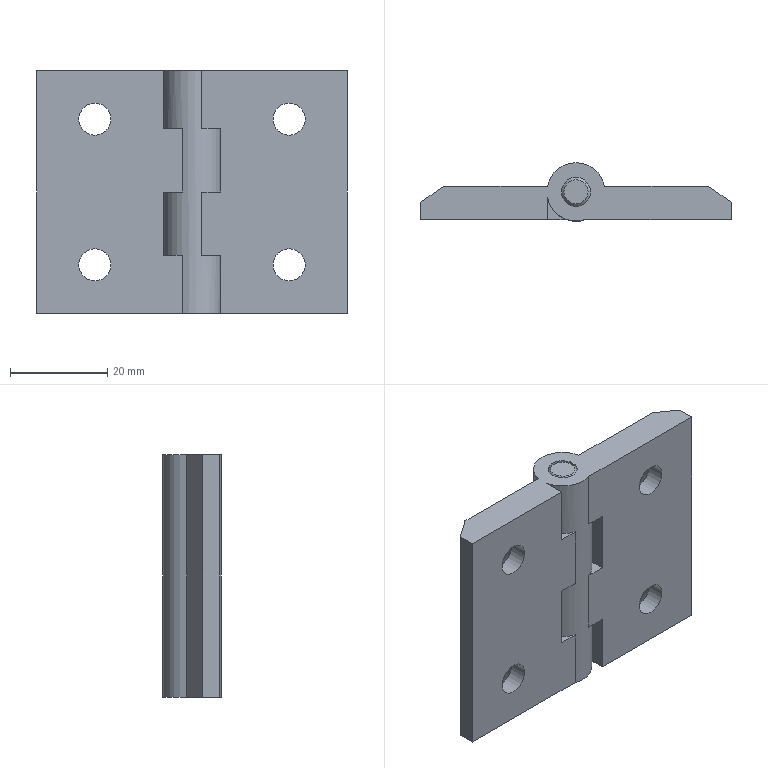Part | STEP file | 40-1-2-SOLID1_id370_x_t | 1 solid | 36 faces | box 64 x 12 x 50 mm | volume 21436 mm3 | plane 22 | cylinder 8 | cone 6 | commonest cylinder face diameters 6.6 x4 6 x2 12 x2
STEP:
#1=CARTESIAN_POINT('',(1872.,280.,-110.));
#2=VERTEX_POINT('',#1);
#3=CARTESIAN_POINT('',(1864.11,284.514,-110.));
#4=VERTEX_POINT('',#3);
#5=CARTESIAN_POINT('',(1870.,285.657,-110.));
#6=DIRECTION('',(0.,0.,-1.));
#7=DIRECTION('',(-1.,0.,0.));
#8=AXIS2_PLACEMENT_3D('',#5,#6,#7);
#9=CIRCLE('',#8,6.);
#10=EDGE_CURVE('',#2,#4,#9,.T.);
#11=ORIENTED_EDGE('',*,*,#10,.T.);
#12=CARTESIAN_POINT('',(1864.11,284.514,-122.));
#13=VERTEX_POINT('',#12);
#14=CARTESIAN_POINT('',(1864.11,284.514,-160.));
#15=DIRECTION('',(0.,0.,-1.));
#16=VECTOR('',#15,1.);
#17=LINE('',#14,#16);
#18=EDGE_CURVE('',#4,#13,#17,.T.);
#19=ORIENTED_EDGE('',*,*,#18,.T.);
#20=CARTESIAN_POINT('',(1868.,280.,-122.));
#21=VERTEX_POINT('',#20);
#22=CARTESIAN_POINT('',(1870.,285.657,-122.));
#23=DIRECTION('',(0.,0.,-1.));
#24=DIRECTION('',(1.,0.,0.));
#25=AXIS2_PLACEMENT_3D('',#22,#23,#24);
#26=CIRCLE('',#25,6.);
#27=EDGE_CURVE('',#21,#13,#26,.T.);
#28=ORIENTED_EDGE('',*,*,#27,.F.);
#29=CARTESIAN_POINT('',(1868.,280.,-135.));
#30=VERTEX_POINT('',#29);
#31=CARTESIAN_POINT('',(1868.,280.,-110.));
#32=DIRECTION('',(0.,0.,1.));
#33=VECTOR('',#32,1.);
#34=LINE('',#31,#33);
#35=EDGE_CURVE('',#30,#21,#34,.T.);
#36=ORIENTED_EDGE('',*,*,#35,.F.);
#37=CARTESIAN_POINT('',(1864.11,284.514,-135.));
#38=VERTEX_POINT('',#37);
#39=CARTESIAN_POINT('',(1870.,285.657,-135.));
#40=DIRECTION('',(0.,0.,-1.));
#41=DIRECTION('',(1.,0.,0.));
#42=AXIS2_PLACEMENT_3D('',#39,#40,#41);
#43=CIRCLE('',#42,6.);
#44=EDGE_CURVE('',#30,#38,#43,.T.);
#45=ORIENTED_EDGE('',*,*,#44,.T.);
#46=CARTESIAN_POINT('',(1864.11,284.514,-148.));
#47=VERTEX_POINT('',#46);
#48=CARTESIAN_POINT('',(1864.11,284.514,-160.));
#49=DIRECTION('',(0.,0.,1.));
#50=VECTOR('',#49,1.);
#51=LINE('',#48,#50);
#52=EDGE_CURVE('',#47,#38,#51,.T.);
#53=ORIENTED_EDGE('',*,*,#52,.F.);
#54=CARTESIAN_POINT('',(1868.,280.,-148.));
#55=VERTEX_POINT('',#54);
#56=CARTESIAN_POINT('',(1870.,285.657,-148.));
#57=DIRECTION('',(0.,0.,-1.));
#58=DIRECTION('',(-1.,0.,0.));
#59=AXIS2_PLACEMENT_3D('',#56,#57,#58);
#60=CIRCLE('',#59,6.);
#61=EDGE_CURVE('',#55,#47,#60,.T.);
#62=ORIENTED_EDGE('',*,*,#61,.F.);
#63=CARTESIAN_POINT('',(1868.,280.,-160.));
#64=VERTEX_POINT('',#63);
#65=CARTESIAN_POINT('',(1868.,280.,-110.));
#66=DIRECTION('',(0.,0.,1.));
#67=VECTOR('',#66,1.);
#68=LINE('',#65,#67);
#69=EDGE_CURVE('',#64,#55,#68,.T.);
#70=ORIENTED_EDGE('',*,*,#69,.F.);
#71=CARTESIAN_POINT('',(1875.89,284.514,-160.));
#72=VERTEX_POINT('',#71);
#73=CARTESIAN_POINT('',(1870.,285.657,-160.));
#74=DIRECTION('',(0.,0.,1.));
#75=DIRECTION('',(1.,0.,0.));
#76=AXIS2_PLACEMENT_3D('',#73,#74,#75);
#77=CIRCLE('',#76,6.);
#78=EDGE_CURVE('',#64,#72,#77,.T.);
#79=ORIENTED_EDGE('',*,*,#78,.T.);
#80=CARTESIAN_POINT('',(1875.89,284.514,-148.));
#81=VERTEX_POINT('',#80);
#82=CARTESIAN_POINT('',(1875.89,284.514,-110.));
#83=DIRECTION('',(0.,0.,-1.));
#84=VECTOR('',#83,1.);
#85=LINE('',#82,#84);
#86=EDGE_CURVE('',#81,#72,#85,.T.);
#87=ORIENTED_EDGE('',*,*,#86,.F.);
#88=CARTESIAN_POINT('',(1872.,280.,-148.));
#89=VERTEX_POINT('',#88);
#90=CARTESIAN_POINT('',(1870.,285.657,-148.));
#91=DIRECTION('',(0.,0.,1.));
#92=DIRECTION('',(1.,0.,0.));
#93=AXIS2_PLACEMENT_3D('',#90,#91,#92);
#94=CIRCLE('',#93,6.);
#95=EDGE_CURVE('',#89,#81,#94,.T.);
#96=ORIENTED_EDGE('',*,*,#95,.F.);
#97=CARTESIAN_POINT('',(1872.,280.,-135.));
#98=VERTEX_POINT('',#97);
#99=CARTESIAN_POINT('',(1872.,280.,-160.));
#100=DIRECTION('',(0.,0.,1.));
#101=VECTOR('',#100,1.);
#102=LINE('',#99,#101);
#103=EDGE_CURVE('',#89,#98,#102,.T.);
#104=ORIENTED_EDGE('',*,*,#103,.T.);
#105=CARTESIAN_POINT('',(1875.89,284.514,-135.));
#106=VERTEX_POINT('',#105);
#107=CARTESIAN_POINT('',(1870.,285.657,-135.));
#108=DIRECTION('',(0.,0.,1.));
#109=DIRECTION('',(-1.,0.,0.));
#110=AXIS2_PLACEMENT_3D('',#107,#108,#109);
#111=CIRCLE('',#110,6.);
#112=EDGE_CURVE('',#98,#106,#111,.T.);
#113=ORIENTED_EDGE('',*,*,#112,.T.);
#114=CARTESIAN_POINT('',(1875.89,284.514,-122.));
#115=VERTEX_POINT('',#114);
#116=CARTESIAN_POINT('',(1875.89,284.514,-110.));
#117=DIRECTION('',(0.,0.,1.));
#118=VECTOR('',#117,1.);
#119=LINE('',#116,#118);
#120=EDGE_CURVE('',#106,#115,#119,.T.);
#121=ORIENTED_EDGE('',*,*,#120,.T.);
#122=CARTESIAN_POINT('',(1872.,280.,-122.));
#123=VERTEX_POINT('',#122);
#124=CARTESIAN_POINT('',(1870.,285.657,-122.));
#125=DIRECTION('',(0.,0.,1.));
#126=DIRECTION('',(1.,0.,0.));
#127=AXIS2_PLACEMENT_3D('',#124,#125,#126);
#128=CIRCLE('',#127,6.);
#129=EDGE_CURVE('',#123,#115,#128,.T.);
#130=ORIENTED_EDGE('',*,*,#129,.F.);
#131=CARTESIAN_POINT('',(1872.,280.,-160.));
#132=DIRECTION('',(0.,0.,1.));
#133=VECTOR('',#132,1.);
#134=LINE('',#131,#133);
#135=EDGE_CURVE('',#123,#2,#134,.T.);
#136=ORIENTED_EDGE('',*,*,#135,.T.);
#137=EDGE_LOOP('',(#11,#19,#28,#36,#45,#53,#62,#70,#79,#87,#96,#104,#113,#121,#130,#136));
#138=FACE_OUTER_BOUND('',#137,.T.);
#139=CARTESIAN_POINT('',(1870.,285.657,-160.));
#140=DIRECTION('',(0.,0.,1.));
#141=DIRECTION('',(-1.,0.,0.));
#142=AXIS2_PLACEMENT_3D('',#139,#140,#141);
#143=CYLINDRICAL_SURFACE('',#142,6.);
#144=ADVANCED_FACE('',(#138),#143,.T.);
#145=CARTESIAN_POINT('',(1864.11,286.8,-160.));
#146=VERTEX_POINT('',#145);
#147=CARTESIAN_POINT('',(1864.11,286.8,-110.));
#148=VERTEX_POINT('',#147);
#149=CARTESIAN_POINT('',(1864.11,286.8,-110.));
#150=DIRECTION('',(0.,0.,1.));
#151=VECTOR('',#150,1.);
#152=LINE('',#149,#151);
#153=EDGE_CURVE('',#146,#148,#152,.T.);
#154=ORIENTED_EDGE('',*,*,#153,.T.);
#155=CARTESIAN_POINT('',(1875.89,286.8,-110.));
#156=VERTEX_POINT('',#155);
#157=CARTESIAN_POINT('',(1870.,285.657,-110.));
#158=DIRECTION('',(0.,0.,-1.));
#159=DIRECTION('',(-1.,0.,0.));
#160=AXIS2_PLACEMENT_3D('',#157,#158,#159);
#161=CIRCLE('',#160,6.);
#162=EDGE_CURVE('',#148,#156,#161,.T.);
#163=ORIENTED_EDGE('',*,*,#162,.T.);
#164=CARTESIAN_POINT('',(1875.89,286.8,-160.));
#165=VERTEX_POINT('',#164);
#166=CARTESIAN_POINT('',(1875.89,286.8,-160.));
#167=DIRECTION('',(0.,0.,1.));
#168=VECTOR('',#167,1.);
#169=LINE('',#166,#168);
#170=EDGE_CURVE('',#165,#156,#169,.T.);
#171=ORIENTED_EDGE('',*,*,#170,.F.);
#172=CARTESIAN_POINT('',(1870.,285.657,-160.));
#173=DIRECTION('',(0.,0.,1.));
#174=DIRECTION('',(1.,0.,0.));
#175=AXIS2_PLACEMENT_3D('',#172,#173,#174);
#176=CIRCLE('',#175,6.);
#177=EDGE_CURVE('',#165,#146,#176,.T.);
#178=ORIENTED_EDGE('',*,*,#177,.T.);
#179=EDGE_LOOP('',(#154,#163,#171,#178));
#180=FACE_OUTER_BOUND('',#179,.T.);
#181=CARTESIAN_POINT('',(1870.,285.657,-160.));
#182=DIRECTION('',(0.,0.,1.));
#183=DIRECTION('',(-1.,0.,0.));
#184=AXIS2_PLACEMENT_3D('',#181,#182,#183);
#185=CYLINDRICAL_SURFACE('',#184,6.);
#186=ADVANCED_FACE('',(#180),#185,.T.);
#187=CARTESIAN_POINT('',(1875.89,280.,-122.));
#188=VERTEX_POINT('',#187);
#189=CARTESIAN_POINT('',(1875.89,280.,-122.));
#190=DIRECTION('',(-1.,0.,0.));
#191=VECTOR('',#190,1.);
#192=LINE('',#189,#191);
#193=EDGE_CURVE('',#188,#123,#192,.T.);
#194=ORIENTED_EDGE('',*,*,#193,.T.);
#195=ORIENTED_EDGE('',*,*,#129,.T.);
#196=CARTESIAN_POINT('',(1875.89,280.,-122.));
#197=DIRECTION('',(0.,1.,0.));
#198=VECTOR('',#197,1.);
#199=LINE('',#196,#198);
#200=EDGE_CURVE('',#188,#115,#199,.T.);
#201=ORIENTED_EDGE('',*,*,#200,.F.);
#202=EDGE_LOOP('',(#194,#195,#201));
#203=FACE_OUTER_BOUND('',#202,.T.);
#204=CARTESIAN_POINT('',(1870.,285.657,-122.));
#205=DIRECTION('',(0.,0.,-1.));
#206=DIRECTION('',(1.,0.,0.));
#207=AXIS2_PLACEMENT_3D('',#204,#205,#206);
#208=PLANE('',#207);
#209=ADVANCED_FACE('',(#203),#208,.T.);
#210=CARTESIAN_POINT('',(1875.89,280.,-148.));
#211=VERTEX_POINT('',#210);
#212=CARTESIAN_POINT('',(1875.89,280.,-148.));
#213=DIRECTION('',(-1.,0.,0.));
#214=VECTOR('',#213,1.);
#215=LINE('',#212,#214);
#216=EDGE_CURVE('',#211,#89,#215,.T.);
#217=ORIENTED_EDGE('',*,*,#216,.T.);
#218=ORIENTED_EDGE('',*,*,#95,.T.);
#219=CARTESIAN_POINT('',(1875.89,285.657,-148.));
#220=DIRECTION('',(0.,-1.,0.));
#221=VECTOR('',#220,1.);
#222=LINE('',#219,#221);
#223=EDGE_CURVE('',#81,#211,#222,.T.);
#224=ORIENTED_EDGE('',*,*,#223,.T.);
#225=EDGE_LOOP('',(#217,#218,#224));
#226=FACE_OUTER_BOUND('',#225,.T.);
#227=CARTESIAN_POINT('',(1870.,285.657,-148.));
#228=DIRECTION('',(0.,0.,-1.));
#229=DIRECTION('',(1.,0.,0.));
#230=AXIS2_PLACEMENT_3D('',#227,#228,#229);
#231=PLANE('',#230);
#232=ADVANCED_FACE('',(#226),#231,.T.);
#233=CARTESIAN_POINT('',(1890.,283.7,-123.3));
#234=VERTEX_POINT('',#233);
#235=CARTESIAN_POINT('',(1890.,283.7,-120.));
#236=DIRECTION('',(0.,1.,0.));
#237=DIRECTION('',(0.,0.,-1.));
#238=AXIS2_PLACEMENT_3D('',#235,#236,#237);
#239=CIRCLE('',#238,3.3);
#240=EDGE_CURVE('',#234,#234,#239,.T.);
#241=ORIENTED_EDGE('',*,*,#240,.F.);
#242=EDGE_LOOP('',(#241));
#243=FACE_BOUND('',#242,.T.);
#244=CARTESIAN_POINT('',(1890.,286.8,-126.4));
#245=VERTEX_POINT('',#244);
#246=CARTESIAN_POINT('',(1890.,286.8,-120.));
#247=DIRECTION('',(0.,1.,0.));
#248=DIRECTION('',(0.,0.,-1.));
#249=AXIS2_PLACEMENT_3D('',#246,#247,#248);
#250=CIRCLE('',#249,6.4);
#251=EDGE_CURVE('',#245,#245,#250,.T.);
#252=ORIENTED_EDGE('',*,*,#251,.T.);
#253=EDGE_LOOP('',(#252));
#254=FACE_BOUND('',#253,.T.);
#255=CARTESIAN_POINT('',(1890.,286.8,-120.));
#256=DIRECTION('',(0.,1.,0.));
#257=DIRECTION('',(0.,0.,1.));
#258=AXIS2_PLACEMENT_3D('',#255,#256,#257);
#259=CONICAL_SURFACE('',#258,6.4,45.);
#260=ADVANCED_FACE('',(#243,#254),#259,.F.);
#261=CARTESIAN_POINT('',(1890.,280.,-116.7));
#262=VERTEX_POINT('',#261);
#263=CARTESIAN_POINT('',(1890.,280.,-120.));
#264=DIRECTION('',(0.,-1.,0.));
#265=DIRECTION('',(0.,0.,1.));
#266=AXIS2_PLACEMENT_3D('',#263,#264,#265);
#267=CIRCLE('',#266,3.3);
#268=EDGE_CURVE('',#262,#262,#267,.T.);
#269=ORIENTED_EDGE('',*,*,#268,.T.);
#270=EDGE_LOOP('',(#269));
#271=FACE_BOUND('',#270,.T.);
#272=ORIENTED_EDGE('',*,*,#240,.T.);
#273=EDGE_LOOP('',(#272));
#274=FACE_BOUND('',#273,.T.);
#275=CARTESIAN_POINT('',(1890.,286.8,-120.));
#276=DIRECTION('',(0.,1.,0.));
#277=DIRECTION('',(0.,0.,1.));
#278=AXIS2_PLACEMENT_3D('',#275,#276,#277);
#279=CYLINDRICAL_SURFACE('',#278,3.3);
#280=ADVANCED_FACE('',(#271,#274),#279,.F.);
#281=CARTESIAN_POINT('',(1890.,283.7,-153.3));
#282=VERTEX_POINT('',#281);
#283=CARTESIAN_POINT('',(1890.,283.7,-150.));
#284=DIRECTION('',(0.,1.,0.));
#285=DIRECTION('',(0.,0.,-1.));
#286=AXIS2_PLACEMENT_3D('',#283,#284,#285);
#287=CIRCLE('',#286,3.3);
#288=EDGE_CURVE('',#282,#282,#287,.T.);
#289=ORIENTED_EDGE('',*,*,#288,.F.);
#290=EDGE_LOOP('',(#289));
#291=FACE_BOUND('',#290,.T.);
#292=CARTESIAN_POINT('',(1890.,286.8,-156.4));
#293=VERTEX_POINT('',#292);
#294=CARTESIAN_POINT('',(1890.,286.8,-150.));
#295=DIRECTION('',(0.,1.,0.));
#296=DIRECTION('',(0.,0.,-1.));
#297=AXIS2_PLACEMENT_3D('',#294,#295,#296);
#298=CIRCLE('',#297,6.4);
#299=EDGE_CURVE('',#293,#293,#298,.T.);
#300=ORIENTED_EDGE('',*,*,#299,.T.);
#301=EDGE_LOOP('',(#300));
#302=FACE_BOUND('',#301,.T.);
#303=CARTESIAN_POINT('',(1890.,286.8,-150.));
#304=DIRECTION('',(0.,1.,0.));
#305=DIRECTION('',(0.,0.,1.));
#306=AXIS2_PLACEMENT_3D('',#303,#304,#305);
#307=CONICAL_SURFACE('',#306,6.4,45.);
#308=ADVANCED_FACE('',(#291,#302),#307,.F.);
#309=CARTESIAN_POINT('',(1890.,280.,-146.7));
#310=VERTEX_POINT('',#309);
#311=CARTESIAN_POINT('',(1890.,280.,-150.));
#312=DIRECTION('',(0.,-1.,0.));
#313=DIRECTION('',(0.,0.,1.));
#314=AXIS2_PLACEMENT_3D('',#311,#312,#313);
#315=CIRCLE('',#314,3.3);
#316=EDGE_CURVE('',#310,#310,#315,.T.);
#317=ORIENTED_EDGE('',*,*,#316,.T.);
#318=EDGE_LOOP('',(#317));
#319=FACE_BOUND('',#318,.T.);
#320=ORIENTED_EDGE('',*,*,#288,.T.);
#321=EDGE_LOOP('',(#320));
#322=FACE_BOUND('',#321,.T.);
#323=CARTESIAN_POINT('',(1890.,286.8,-150.));
#324=DIRECTION('',(0.,1.,0.));
#325=DIRECTION('',(0.,0.,1.));
#326=AXIS2_PLACEMENT_3D('',#323,#324,#325);
#327=CYLINDRICAL_SURFACE('',#326,3.3);
#328=ADVANCED_FACE('',(#319,#322),#327,.F.);
#329=CARTESIAN_POINT('',(1873.,285.657,-110.5));
#330=VERTEX_POINT('',#329);
#331=CARTESIAN_POINT('',(1870.,285.657,-110.5));
#332=DIRECTION('',(0.,0.,-1.));
#333=DIRECTION('',(1.,0.,0.));
#334=AXIS2_PLACEMENT_3D('',#331,#332,#333);
#335=CIRCLE('',#334,3.);
#336=EDGE_CURVE('',#330,#330,#335,.T.);
#337=ORIENTED_EDGE('',*,*,#336,.T.);
#338=EDGE_LOOP('',(#337));
#339=FACE_BOUND('',#338,.T.);
#340=CARTESIAN_POINT('',(1867.,285.657,-110.));
#341=VERTEX_POINT('',#340);
#342=CARTESIAN_POINT('',(1870.,285.657,-110.));
#343=DIRECTION('',(0.,0.,-1.));
#344=DIRECTION('',(-1.,0.,0.));
#345=AXIS2_PLACEMENT_3D('',#342,#343,#344);
#346=CIRCLE('',#345,3.);
#347=EDGE_CURVE('',#341,#341,#346,.T.);
#348=ORIENTED_EDGE('',*,*,#347,.F.);
#349=EDGE_LOOP('',(#348));
#350=FACE_BOUND('',#349,.T.);
#351=CARTESIAN_POINT('',(1870.,285.657,-122.));
#352=DIRECTION('',(0.,0.,-1.));
#353=DIRECTION('',(1.,0.,0.));
#354=AXIS2_PLACEMENT_3D('',#351,#352,#353);
#355=CYLINDRICAL_SURFACE('',#354,3.);
#356=ADVANCED_FACE('',(#339,#350),#355,.F.);
#357=ORIENTED_EDGE('',*,*,#251,.F.);
#358=EDGE_LOOP('',(#357));
#359=FACE_BOUND('',#358,.T.);
#360=ORIENTED_EDGE('',*,*,#299,.F.);
#361=EDGE_LOOP('',(#360));
#362=FACE_BOUND('',#361,.T.);
#363=CARTESIAN_POINT('',(1897.287,286.8,-110.));
#364=VERTEX_POINT('',#363);
#365=CARTESIAN_POINT('',(1897.287,286.8,-160.));
#366=VERTEX_POINT('',#365);
#367=CARTESIAN_POINT('',(1897.287,286.8,-110.));
#368=DIRECTION('',(0.,0.,-1.));
#369=VECTOR('',#368,1.);
#370=LINE('',#367,#369);
#371=EDGE_CURVE('',#364,#366,#370,.T.);
#372=ORIENTED_EDGE('',*,*,#371,.T.);
#373=CARTESIAN_POINT('',(1897.287,286.8,-160.));
#374=DIRECTION('',(1.,0.,0.));
#375=VECTOR('',#374,1.);
#376=LINE('',#373,#375);
#377=EDGE_CURVE('',#165,#366,#376,.T.);
#378=ORIENTED_EDGE('',*,*,#377,.F.);
#379=ORIENTED_EDGE('',*,*,#170,.T.);
#380=CARTESIAN_POINT('',(1875.89,286.8,-110.));
#381=DIRECTION('',(1.,0.,0.));
#382=VECTOR('',#381,1.);
#383=LINE('',#380,#382);
#384=EDGE_CURVE('',#156,#364,#383,.T.);
#385=ORIENTED_EDGE('',*,*,#384,.T.);
#386=EDGE_LOOP('',(#372,#378,#379,#385));
#387=FACE_BOUND('',#386,.T.);
#388=CARTESIAN_POINT('',(1875.89,286.8,-110.));
#389=DIRECTION('',(0.,1.,0.));
#390=DIRECTION('',(0.,0.,1.));
#391=AXIS2_PLACEMENT_3D('',#388,#389,#390);
#392=PLANE('',#391);
#393=ADVANCED_FACE('',(#359,#362,#387),#392,.T.);
#394=ORIENTED_EDGE('',*,*,#268,.F.);
#395=EDGE_LOOP('',(#394));
#396=FACE_BOUND('',#395,.T.);
#397=ORIENTED_EDGE('',*,*,#316,.F.);
#398=EDGE_LOOP('',(#397));
#399=FACE_BOUND('',#398,.T.);
#400=CARTESIAN_POINT('',(1875.89,280.,-160.));
#401=VERTEX_POINT('',#400);
#402=CARTESIAN_POINT('',(1875.89,280.,-110.));
#403=DIRECTION('',(0.,0.,-1.));
#404=VECTOR('',#403,1.);
#405=LINE('',#402,#404);
#406=EDGE_CURVE('',#211,#401,#405,.T.);
#407=ORIENTED_EDGE('',*,*,#406,.T.);
#408=CARTESIAN_POINT('',(1902.,280.,-160.));
#409=VERTEX_POINT('',#408);
#410=CARTESIAN_POINT('',(1872.,280.,-160.));
#411=DIRECTION('',(-1.,0.,0.));
#412=VECTOR('',#411,1.);
#413=LINE('',#410,#412);
#414=EDGE_CURVE('',#409,#401,#413,.T.);
#415=ORIENTED_EDGE('',*,*,#414,.F.);
#416=CARTESIAN_POINT('',(1902.,280.,-110.));
#417=VERTEX_POINT('',#416);
#418=CARTESIAN_POINT('',(1902.,280.,-110.));
#419=DIRECTION('',(0.,0.,-1.));
#420=VECTOR('',#419,1.);
#421=LINE('',#418,#420);
#422=EDGE_CURVE('',#417,#409,#421,.T.);
#423=ORIENTED_EDGE('',*,*,#422,.F.);
#424=CARTESIAN_POINT('',(1902.,280.,-110.));
#425=DIRECTION('',(-1.,0.,0.));
#426=VECTOR('',#425,1.);
#427=LINE('',#424,#426);
#428=EDGE_CURVE('',#417,#2,#427,.T.);
#429=ORIENTED_EDGE('',*,*,#428,.T.);
#430=ORIENTED_EDGE('',*,*,#135,.F.);
#431=ORIENTED_EDGE('',*,*,#193,.F.);
#432=CARTESIAN_POINT('',(1875.89,280.,-135.));
#433=VERTEX_POINT('',#432);
#434=CARTESIAN_POINT('',(1875.89,280.,-135.));
#435=DIRECTION('',(0.,0.,1.));
#436=VECTOR('',#435,1.);
#437=LINE('',#434,#436);
#438=EDGE_CURVE('',#433,#188,#437,.T.);
#439=ORIENTED_EDGE('',*,*,#438,.F.);
#440=CARTESIAN_POINT('',(1872.,280.,-135.));
#441=DIRECTION('',(-1.,0.,0.));
#442=VECTOR('',#441,1.);
#443=LINE('',#440,#442);
#444=EDGE_CURVE('',#433,#98,#443,.T.);
#445=ORIENTED_EDGE('',*,*,#444,.T.);
#446=ORIENTED_EDGE('',*,*,#103,.F.);
#447=ORIENTED_EDGE('',*,*,#216,.F.);
#448=EDGE_LOOP('',(#407,#415,#423,#429,#430,#431,#439,#445,#446,#447));
#449=FACE_BOUND('',#448,.T.);
#450=CARTESIAN_POINT('',(1902.,280.,-110.));
#451=DIRECTION('',(0.,-1.,0.));
#452=DIRECTION('',(0.,0.,-1.));
#453=AXIS2_PLACEMENT_3D('',#450,#451,#452);
#454=PLANE('',#453);
#455=ADVANCED_FACE('',(#396,#399,#449),#454,.T.);
#456=ORIENTED_EDGE('',*,*,#422,.T.);
#457=CARTESIAN_POINT('',(1902.,283.5,-160.));
#458=VERTEX_POINT('',#457);
#459=CARTESIAN_POINT('',(1902.,280.,-160.));
#460=DIRECTION('',(0.,-1.,0.));
#461=VECTOR('',#460,1.);
#462=LINE('',#459,#461);
#463=EDGE_CURVE('',#458,#409,#462,.T.);
#464=ORIENTED_EDGE('',*,*,#463,.F.);
#465=CARTESIAN_POINT('',(1902.,283.5,-110.));
#466=VERTEX_POINT('',#465);
#467=CARTESIAN_POINT('',(1902.,283.5,-110.));
#468=DIRECTION('',(0.,0.,-1.));
#469=VECTOR('',#468,1.);
#470=LINE('',#467,#469);
#471=EDGE_CURVE('',#466,#458,#470,.T.);
#472=ORIENTED_EDGE('',*,*,#471,.F.);
#473=CARTESIAN_POINT('',(1902.,283.5,-110.));
#474=DIRECTION('',(0.,-1.,0.));
#475=VECTOR('',#474,1.);
#476=LINE('',#473,#475);
#477=EDGE_CURVE('',#466,#417,#476,.T.);
#478=ORIENTED_EDGE('',*,*,#477,.T.);
#479=EDGE_LOOP('',(#456,#464,#472,#478));
#480=FACE_OUTER_BOUND('',#479,.T.);
#481=CARTESIAN_POINT('',(1902.,283.5,-110.));
#482=DIRECTION('',(1.,0.,0.));
#483=DIRECTION('',(0.,1.,0.));
#484=AXIS2_PLACEMENT_3D('',#481,#482,#483);
#485=PLANE('',#484);
#486=ADVANCED_FACE('',(#480),#485,.T.);
#487=ORIENTED_EDGE('',*,*,#471,.T.);
#488=CARTESIAN_POINT('',(1902.,283.5,-160.));
#489=DIRECTION('',(0.8192,-0.5736,0.));
#490=VECTOR('',#489,1.);
#491=LINE('',#488,#490);
#492=EDGE_CURVE('',#366,#458,#491,.T.);
#493=ORIENTED_EDGE('',*,*,#492,.F.);
#494=ORIENTED_EDGE('',*,*,#371,.F.);
#495=CARTESIAN_POINT('',(1897.287,286.8,-110.));
#496=DIRECTION('',(0.8192,-0.5736,0.));
#497=VECTOR('',#496,1.);
#498=LINE('',#495,#497);
#499=EDGE_CURVE('',#364,#466,#498,.T.);
#500=ORIENTED_EDGE('',*,*,#499,.T.);
#501=EDGE_LOOP('',(#487,#493,#494,#500));
#502=FACE_OUTER_BOUND('',#501,.T.);
#503=CARTESIAN_POINT('',(1897.287,286.8,-110.));
#504=DIRECTION('',(0.5736,0.8192,0.));
#505=DIRECTION('',(-0.8192,0.5736,0.));
#506=AXIS2_PLACEMENT_3D('',#503,#504,#505);
#507=PLANE('',#506);
#508=ADVANCED_FACE('',(#502),#507,.T.);
#509=ORIENTED_EDGE('',*,*,#347,.T.);
#510=EDGE_LOOP('',(#509));
#511=FACE_BOUND('',#510,.T.);
#512=ORIENTED_EDGE('',*,*,#162,.F.);
#513=CARTESIAN_POINT('',(1842.713,286.8,-110.));
#514=VERTEX_POINT('',#513);
#515=CARTESIAN_POINT('',(1842.713,286.8,-110.));
#516=DIRECTION('',(-1.,0.,0.));
#517=VECTOR('',#516,1.);
#518=LINE('',#515,#517);
#519=EDGE_CURVE('',#148,#514,#518,.T.);
#520=ORIENTED_EDGE('',*,*,#519,.T.);
#521=CARTESIAN_POINT('',(1838.,283.5,-110.));
#522=VERTEX_POINT('',#521);
#523=CARTESIAN_POINT('',(1838.,283.5,-110.));
#524=DIRECTION('',(-0.8192,-0.5736,0.));
#525=VECTOR('',#524,1.);
#526=LINE('',#523,#525);
#527=EDGE_CURVE('',#514,#522,#526,.T.);
#528=ORIENTED_EDGE('',*,*,#527,.T.);
#529=CARTESIAN_POINT('',(1838.,280.,-110.));
#530=VERTEX_POINT('',#529);
#531=CARTESIAN_POINT('',(1838.,280.,-110.));
#532=DIRECTION('',(0.,-1.,0.));
#533=VECTOR('',#532,1.);
#534=LINE('',#531,#533);
#535=EDGE_CURVE('',#522,#530,#534,.T.);
#536=ORIENTED_EDGE('',*,*,#535,.T.);
#537=CARTESIAN_POINT('',(1864.11,280.,-110.));
#538=VERTEX_POINT('',#537);
#539=CARTESIAN_POINT('',(1868.,280.,-110.));
#540=DIRECTION('',(1.,0.,0.));
#541=VECTOR('',#540,1.);
#542=LINE('',#539,#541);
#543=EDGE_CURVE('',#530,#538,#542,.T.);
#544=ORIENTED_EDGE('',*,*,#543,.T.);
#545=CARTESIAN_POINT('',(1864.11,280.,-110.));
#546=DIRECTION('',(0.,-1.,0.));
#547=VECTOR('',#546,1.);
#548=LINE('',#545,#547);
#549=EDGE_CURVE('',#4,#538,#548,.T.);
#550=ORIENTED_EDGE('',*,*,#549,.F.);
#551=ORIENTED_EDGE('',*,*,#10,.F.);
#552=ORIENTED_EDGE('',*,*,#428,.F.);
#553=ORIENTED_EDGE('',*,*,#477,.F.);
#554=ORIENTED_EDGE('',*,*,#499,.F.);
#555=ORIENTED_EDGE('',*,*,#384,.F.);
#556=EDGE_LOOP('',(#512,#520,#528,#536,#544,#550,#551,#552,#553,#554,#555));
#557=FACE_BOUND('',#556,.T.);
#558=CARTESIAN_POINT('',(1870.,285.657,-110.));
#559=DIRECTION('',(0.,0.,-1.));
#560=DIRECTION('',(1.,0.,0.));
#561=AXIS2_PLACEMENT_3D('',#558,#559,#560);
#562=PLANE('',#561);
#563=ADVANCED_FACE('',(#511,#557),#562,.F.);
#564=ORIENTED_EDGE('',*,*,#120,.F.);
#565=CARTESIAN_POINT('',(1875.89,286.8,-135.));
#566=DIRECTION('',(0.,-1.,0.));
#567=VECTOR('',#566,1.);
#568=LINE('',#565,#567);
#569=EDGE_CURVE('',#106,#433,#568,.T.);
#570=ORIENTED_EDGE('',*,*,#569,.T.);
#571=ORIENTED_EDGE('',*,*,#438,.T.);
#572=ORIENTED_EDGE('',*,*,#200,.T.);
#573=EDGE_LOOP('',(#564,#570,#571,#572));
#574=FACE_OUTER_BOUND('',#573,.T.);
#575=CARTESIAN_POINT('',(1875.89,280.,-110.));
#576=DIRECTION('',(-1.,0.,0.));
#577=DIRECTION('',(0.,-1.,0.));
#578=AXIS2_PLACEMENT_3D('',#575,#576,#577);
#579=PLANE('',#578);
#580=ADVANCED_FACE('',(#574),#579,.T.);
#581=ORIENTED_EDGE('',*,*,#112,.F.);
#582=ORIENTED_EDGE('',*,*,#444,.F.);
#583=ORIENTED_EDGE('',*,*,#569,.F.);
#584=EDGE_LOOP('',(#581,#582,#583));
#585=FACE_OUTER_BOUND('',#584,.T.);
#586=CARTESIAN_POINT('',(1870.,285.657,-135.));
#587=DIRECTION('',(0.,0.,1.));
#588=DIRECTION('',(-1.,0.,0.));
#589=AXIS2_PLACEMENT_3D('',#586,#587,#588);
#590=PLANE('',#589);
#591=ADVANCED_FACE('',(#585),#590,.T.);
#592=CARTESIAN_POINT('',(1875.89,280.,-160.));
#593=DIRECTION('',(0.,-1.,0.));
#594=VECTOR('',#593,1.);
#595=LINE('',#592,#594);
#596=EDGE_CURVE('',#72,#401,#595,.T.);
#597=ORIENTED_EDGE('',*,*,#596,.F.);
#598=ORIENTED_EDGE('',*,*,#78,.F.);
#599=CARTESIAN_POINT('',(1838.,280.,-160.));
#600=VERTEX_POINT('',#599);
#601=CARTESIAN_POINT('',(1838.,280.,-160.));
#602=DIRECTION('',(1.,0.,0.));
#603=VECTOR('',#602,1.);
#604=LINE('',#601,#603);
#605=EDGE_CURVE('',#600,#64,#604,.T.);
#606=ORIENTED_EDGE('',*,*,#605,.F.);
#607=CARTESIAN_POINT('',(1838.,283.5,-160.));
#608=VERTEX_POINT('',#607);
#609=CARTESIAN_POINT('',(1838.,283.5,-160.));
#610=DIRECTION('',(0.,-1.,0.));
#611=VECTOR('',#610,1.);
#612=LINE('',#609,#611);
#613=EDGE_CURVE('',#608,#600,#612,.T.);
#614=ORIENTED_EDGE('',*,*,#613,.F.);
#615=CARTESIAN_POINT('',(1842.713,286.8,-160.));
#616=VERTEX_POINT('',#615);
#617=CARTESIAN_POINT('',(1842.713,286.8,-160.));
#618=DIRECTION('',(-0.8192,-0.5736,0.));
#619=VECTOR('',#618,1.);
#620=LINE('',#617,#619);
#621=EDGE_CURVE('',#616,#608,#620,.T.);
#622=ORIENTED_EDGE('',*,*,#621,.F.);
#623=CARTESIAN_POINT('',(1864.11,286.8,-160.));
#624=DIRECTION('',(-1.,0.,0.));
#625=VECTOR('',#624,1.);
#626=LINE('',#623,#625);
#627=EDGE_CURVE('',#146,#616,#626,.T.);
#628=ORIENTED_EDGE('',*,*,#627,.F.);
#629=ORIENTED_EDGE('',*,*,#177,.F.);
#630=ORIENTED_EDGE('',*,*,#377,.T.);
#631=ORIENTED_EDGE('',*,*,#492,.T.);
#632=ORIENTED_EDGE('',*,*,#463,.T.);
#633=ORIENTED_EDGE('',*,*,#414,.T.);
#634=EDGE_LOOP('',(#597,#598,#606,#614,#622,#628,#629,#630,#631,#632,#633));
#635=FACE_BOUND('',#634,.T.);
#636=CARTESIAN_POINT('',(1873.,285.657,-160.));
#637=VERTEX_POINT('',#636);
#638=CARTESIAN_POINT('',(1870.,285.657,-160.));
#639=DIRECTION('',(0.,0.,1.));
#640=DIRECTION('',(1.,0.,0.));
#641=AXIS2_PLACEMENT_3D('',#638,#639,#640);
#642=CIRCLE('',#641,3.);
#643=EDGE_CURVE('',#637,#637,#642,.T.);
#644=ORIENTED_EDGE('',*,*,#643,.T.);
#645=EDGE_LOOP('',(#644));
#646=FACE_BOUND('',#645,.T.);
#647=CARTESIAN_POINT('',(1870.,285.657,-160.));
#648=DIRECTION('',(0.,0.,1.));
#649=DIRECTION('',(-1.,0.,0.));
#650=AXIS2_PLACEMENT_3D('',#647,#648,#649);
#651=PLANE('',#650);
#652=ADVANCED_FACE('',(#635,#646),#651,.F.);
#653=ORIENTED_EDGE('',*,*,#223,.F.);
#654=ORIENTED_EDGE('',*,*,#86,.T.);
#655=ORIENTED_EDGE('',*,*,#596,.T.);
#656=ORIENTED_EDGE('',*,*,#406,.F.);
#657=EDGE_LOOP('',(#653,#654,#655,#656));
#658=FACE_OUTER_BOUND('',#657,.T.);
#659=CARTESIAN_POINT('',(1875.89,280.,-110.));
#660=DIRECTION('',(-1.,0.,0.));
#661=DIRECTION('',(0.,-1.,0.));
#662=AXIS2_PLACEMENT_3D('',#659,#660,#661);
#663=PLANE('',#662);
#664=ADVANCED_FACE('',(#658),#663,.T.);
#665=CARTESIAN_POINT('',(1872.5,285.657,-160.));
#666=VERTEX_POINT('',#665);
#667=CARTESIAN_POINT('',(1870.,285.657,-160.));
#668=DIRECTION('',(0.,0.,-1.));
#669=DIRECTION('',(1.,0.,0.));
#670=AXIS2_PLACEMENT_3D('',#667,#668,#669);
#671=CIRCLE('',#670,2.5);
#672=EDGE_CURVE('',#666,#666,#671,.T.);
#673=ORIENTED_EDGE('',*,*,#672,.F.);
#674=EDGE_LOOP('',(#673));
#675=FACE_BOUND('',#674,.T.);
#676=CARTESIAN_POINT('',(1873.,285.657,-159.5));
#677=VERTEX_POINT('',#676);
#678=CARTESIAN_POINT('',(1870.,285.657,-159.5));
#679=DIRECTION('',(0.,0.,1.));
#680=DIRECTION('',(1.,0.,0.));
#681=AXIS2_PLACEMENT_3D('',#678,#679,#680);
#682=CIRCLE('',#681,3.);
#683=EDGE_CURVE('',#677,#677,#682,.T.);
#684=ORIENTED_EDGE('',*,*,#683,.F.);
#685=EDGE_LOOP('',(#684));
#686=FACE_BOUND('',#685,.T.);
#687=CARTESIAN_POINT('',(1870.,285.657,-159.5));
#688=DIRECTION('',(0.,0.,1.));
#689=DIRECTION('',(1.,0.,0.));
#690=AXIS2_PLACEMENT_3D('',#687,#688,#689);
#691=CONICAL_SURFACE('',#690,3.,45.);
#692=ADVANCED_FACE('',(#675,#686),#691,.T.);
#693=ORIENTED_EDGE('',*,*,#672,.T.);
#694=EDGE_LOOP('',(#693));
#695=FACE_OUTER_BOUND('',#694,.T.);
#696=CARTESIAN_POINT('',(1870.,285.657,-160.));
#697=DIRECTION('',(0.,0.,1.));
#698=DIRECTION('',(-1.,0.,0.));
#699=AXIS2_PLACEMENT_3D('',#696,#697,#698);
#700=PLANE('',#699);
#701=ADVANCED_FACE('',(#695),#700,.F.);
#702=CARTESIAN_POINT('',(1864.11,280.,-122.));
#703=VERTEX_POINT('',#702);
#704=CARTESIAN_POINT('',(1864.11,280.,-122.));
#705=DIRECTION('',(1.,0.,0.));
#706=VECTOR('',#705,1.);
#707=LINE('',#704,#706);
#708=EDGE_CURVE('',#703,#21,#707,.T.);
#709=ORIENTED_EDGE('',*,*,#708,.T.);
#710=ORIENTED_EDGE('',*,*,#27,.T.);
#711=CARTESIAN_POINT('',(1864.11,285.657,-122.));
#712=DIRECTION('',(0.,-1.,0.));
#713=VECTOR('',#712,1.);
#714=LINE('',#711,#713);
#715=EDGE_CURVE('',#13,#703,#714,.T.);
#716=ORIENTED_EDGE('',*,*,#715,.T.);
#717=EDGE_LOOP('',(#709,#710,#716));
#718=FACE_OUTER_BOUND('',#717,.T.);
#719=CARTESIAN_POINT('',(1870.,285.657,-122.));
#720=DIRECTION('',(0.,0.,1.));
#721=DIRECTION('',(-1.,0.,0.));
#722=AXIS2_PLACEMENT_3D('',#719,#720,#721);
#723=PLANE('',#722);
#724=ADVANCED_FACE('',(#718),#723,.T.);
#725=ORIENTED_EDGE('',*,*,#18,.F.);
#726=ORIENTED_EDGE('',*,*,#549,.T.);
#727=CARTESIAN_POINT('',(1864.11,280.,-160.));
#728=DIRECTION('',(0.,0.,1.));
#729=VECTOR('',#728,1.);
#730=LINE('',#727,#729);
#731=EDGE_CURVE('',#703,#538,#730,.T.);
#732=ORIENTED_EDGE('',*,*,#731,.F.);
#733=ORIENTED_EDGE('',*,*,#715,.F.);
#734=EDGE_LOOP('',(#725,#726,#732,#733));
#735=FACE_OUTER_BOUND('',#734,.T.);
#736=CARTESIAN_POINT('',(1864.11,280.,-160.));
#737=DIRECTION('',(1.,0.,0.));
#738=DIRECTION('',(0.,-1.,0.));
#739=AXIS2_PLACEMENT_3D('',#736,#737,#738);
#740=PLANE('',#739);
#741=ADVANCED_FACE('',(#735),#740,.T.);
#742=CARTESIAN_POINT('',(1864.11,280.,-135.));
#743=VERTEX_POINT('',#742);
#744=CARTESIAN_POINT('',(1864.11,286.8,-135.));
#745=DIRECTION('',(0.,-1.,0.));
#746=VECTOR('',#745,1.);
#747=LINE('',#744,#746);
#748=EDGE_CURVE('',#38,#743,#747,.T.);
#749=ORIENTED_EDGE('',*,*,#748,.F.);
#750=ORIENTED_EDGE('',*,*,#44,.F.);
#751=CARTESIAN_POINT('',(1868.,280.,-135.));
#752=DIRECTION('',(1.,0.,0.));
#753=VECTOR('',#752,1.);
#754=LINE('',#751,#753);
#755=EDGE_CURVE('',#743,#30,#754,.T.);
#756=ORIENTED_EDGE('',*,*,#755,.F.);
#757=EDGE_LOOP('',(#749,#750,#756));
#758=FACE_OUTER_BOUND('',#757,.T.);
#759=CARTESIAN_POINT('',(1870.,285.657,-135.));
#760=DIRECTION('',(0.,0.,-1.));
#761=DIRECTION('',(1.,0.,0.));
#762=AXIS2_PLACEMENT_3D('',#759,#760,#761);
#763=PLANE('',#762);
#764=ADVANCED_FACE('',(#758),#763,.T.);
#765=CARTESIAN_POINT('',(1864.11,280.,-148.));
#766=VERTEX_POINT('',#765);
#767=CARTESIAN_POINT('',(1864.11,280.,-148.));
#768=DIRECTION('',(0.,1.,0.));
#769=VECTOR('',#768,1.);
#770=LINE('',#767,#769);
#771=EDGE_CURVE('',#766,#47,#770,.T.);
#772=ORIENTED_EDGE('',*,*,#771,.T.);
#773=ORIENTED_EDGE('',*,*,#52,.T.);
#774=ORIENTED_EDGE('',*,*,#748,.T.);
#775=CARTESIAN_POINT('',(1864.11,280.,-135.));
#776=DIRECTION('',(0.,0.,-1.));
#777=VECTOR('',#776,1.);
#778=LINE('',#775,#777);
#779=EDGE_CURVE('',#743,#766,#778,.T.);
#780=ORIENTED_EDGE('',*,*,#779,.T.);
#781=EDGE_LOOP('',(#772,#773,#774,#780));
#782=FACE_OUTER_BOUND('',#781,.T.);
#783=CARTESIAN_POINT('',(1864.11,280.,-160.));
#784=DIRECTION('',(1.,0.,0.));
#785=DIRECTION('',(0.,-1.,0.));
#786=AXIS2_PLACEMENT_3D('',#783,#784,#785);
#787=PLANE('',#786);
#788=ADVANCED_FACE('',(#782),#787,.T.);
#789=CARTESIAN_POINT('',(1864.11,280.,-148.));
#790=DIRECTION('',(1.,0.,0.));
#791=VECTOR('',#790,1.);
#792=LINE('',#789,#791);
#793=EDGE_CURVE('',#766,#55,#792,.T.);
#794=ORIENTED_EDGE('',*,*,#793,.T.);
#795=ORIENTED_EDGE('',*,*,#61,.T.);
#796=ORIENTED_EDGE('',*,*,#771,.F.);
#797=EDGE_LOOP('',(#794,#795,#796));
#798=FACE_OUTER_BOUND('',#797,.T.);
#799=CARTESIAN_POINT('',(1870.,285.657,-148.));
#800=DIRECTION('',(0.,0.,1.));
#801=DIRECTION('',(-1.,0.,0.));
#802=AXIS2_PLACEMENT_3D('',#799,#800,#801);
#803=PLANE('',#802);
#804=ADVANCED_FACE('',(#798),#803,.T.);
#805=CARTESIAN_POINT('',(1838.,283.5,-160.));
#806=DIRECTION('',(0.,0.,1.));
#807=VECTOR('',#806,1.);
#808=LINE('',#805,#807);
#809=EDGE_CURVE('',#608,#522,#808,.T.);
#810=ORIENTED_EDGE('',*,*,#809,.T.);
#811=ORIENTED_EDGE('',*,*,#527,.F.);
#812=CARTESIAN_POINT('',(1842.713,286.8,-160.));
#813=DIRECTION('',(0.,0.,1.));
#814=VECTOR('',#813,1.);
#815=LINE('',#812,#814);
#816=EDGE_CURVE('',#616,#514,#815,.T.);
#817=ORIENTED_EDGE('',*,*,#816,.F.);
#818=ORIENTED_EDGE('',*,*,#621,.T.);
#819=EDGE_LOOP('',(#810,#811,#817,#818));
#820=FACE_OUTER_BOUND('',#819,.T.);
#821=CARTESIAN_POINT('',(1842.713,286.8,-160.));
#822=DIRECTION('',(-0.5736,0.8192,0.));
#823=DIRECTION('',(0.8192,0.5736,0.));
#824=AXIS2_PLACEMENT_3D('',#821,#822,#823);
#825=PLANE('',#824);
#826=ADVANCED_FACE('',(#820),#825,.T.);
#827=CARTESIAN_POINT('',(1838.,280.,-160.));
#828=DIRECTION('',(0.,0.,1.));
#829=VECTOR('',#828,1.);
#830=LINE('',#827,#829);
#831=EDGE_CURVE('',#600,#530,#830,.T.);
#832=ORIENTED_EDGE('',*,*,#831,.T.);
#833=ORIENTED_EDGE('',*,*,#535,.F.);
#834=ORIENTED_EDGE('',*,*,#809,.F.);
#835=ORIENTED_EDGE('',*,*,#613,.T.);
#836=EDGE_LOOP('',(#832,#833,#834,#835));
#837=FACE_OUTER_BOUND('',#836,.T.);
#838=CARTESIAN_POINT('',(1838.,283.5,-160.));
#839=DIRECTION('',(-1.,0.,0.));
#840=DIRECTION('',(0.,1.,0.));
#841=AXIS2_PLACEMENT_3D('',#838,#839,#840);
#842=PLANE('',#841);
#843=ADVANCED_FACE('',(#837),#842,.T.);
#844=CARTESIAN_POINT('',(1850.,280.,-153.3));
#845=VERTEX_POINT('',#844);
#846=CARTESIAN_POINT('',(1850.,280.,-150.));
#847=DIRECTION('',(0.,-1.,0.));
#848=DIRECTION('',(0.,0.,-1.));
#849=AXIS2_PLACEMENT_3D('',#846,#847,#848);
#850=CIRCLE('',#849,3.3);
#851=EDGE_CURVE('',#845,#845,#850,.T.);
#852=ORIENTED_EDGE('',*,*,#851,.F.);
#853=EDGE_LOOP('',(#852));
#854=FACE_BOUND('',#853,.T.);
#855=CARTESIAN_POINT('',(1850.,280.,-123.3));
#856=VERTEX_POINT('',#855);
#857=CARTESIAN_POINT('',(1850.,280.,-120.));
#858=DIRECTION('',(0.,-1.,0.));
#859=DIRECTION('',(0.,0.,-1.));
#860=AXIS2_PLACEMENT_3D('',#857,#858,#859);
#861=CIRCLE('',#860,3.3);
#862=EDGE_CURVE('',#856,#856,#861,.T.);
#863=ORIENTED_EDGE('',*,*,#862,.F.);
#864=EDGE_LOOP('',(#863));
#865=FACE_BOUND('',#864,.T.);
#866=ORIENTED_EDGE('',*,*,#731,.T.);
#867=ORIENTED_EDGE('',*,*,#543,.F.);
#868=ORIENTED_EDGE('',*,*,#831,.F.);
#869=ORIENTED_EDGE('',*,*,#605,.T.);
#870=ORIENTED_EDGE('',*,*,#69,.T.);
#871=ORIENTED_EDGE('',*,*,#793,.F.);
#872=ORIENTED_EDGE('',*,*,#779,.F.);
#873=ORIENTED_EDGE('',*,*,#755,.T.);
#874=ORIENTED_EDGE('',*,*,#35,.T.);
#875=ORIENTED_EDGE('',*,*,#708,.F.);
#876=EDGE_LOOP('',(#866,#867,#868,#869,#870,#871,#872,#873,#874,#875));
#877=FACE_BOUND('',#876,.T.);
#878=CARTESIAN_POINT('',(1838.,280.,-160.));
#879=DIRECTION('',(0.,-1.,0.));
#880=DIRECTION('',(0.,0.,1.));
#881=AXIS2_PLACEMENT_3D('',#878,#879,#880);
#882=PLANE('',#881);
#883=ADVANCED_FACE('',(#854,#865,#877),#882,.T.);
#884=CARTESIAN_POINT('',(1850.,286.8,-143.6));
#885=VERTEX_POINT('',#884);
#886=CARTESIAN_POINT('',(1850.,286.8,-150.));
#887=DIRECTION('',(0.,1.,0.));
#888=DIRECTION('',(0.,0.,1.));
#889=AXIS2_PLACEMENT_3D('',#886,#887,#888);
#890=CIRCLE('',#889,6.4);
#891=EDGE_CURVE('',#885,#885,#890,.T.);
#892=ORIENTED_EDGE('',*,*,#891,.F.);
#893=EDGE_LOOP('',(#892));
#894=FACE_BOUND('',#893,.T.);
#895=CARTESIAN_POINT('',(1850.,286.8,-113.6));
#896=VERTEX_POINT('',#895);
#897=CARTESIAN_POINT('',(1850.,286.8,-120.));
#898=DIRECTION('',(0.,1.,0.));
#899=DIRECTION('',(0.,0.,1.));
#900=AXIS2_PLACEMENT_3D('',#897,#898,#899);
#901=CIRCLE('',#900,6.4);
#902=EDGE_CURVE('',#896,#896,#901,.T.);
#903=ORIENTED_EDGE('',*,*,#902,.F.);
#904=EDGE_LOOP('',(#903));
#905=FACE_BOUND('',#904,.T.);
#906=ORIENTED_EDGE('',*,*,#816,.T.);
#907=ORIENTED_EDGE('',*,*,#519,.F.);
#908=ORIENTED_EDGE('',*,*,#153,.F.);
#909=ORIENTED_EDGE('',*,*,#627,.T.);
#910=EDGE_LOOP('',(#906,#907,#908,#909));
#911=FACE_BOUND('',#910,.T.);
#912=CARTESIAN_POINT('',(1864.11,286.8,-160.));
#913=DIRECTION('',(0.,1.,0.));
#914=DIRECTION('',(0.,0.,-1.));
#915=AXIS2_PLACEMENT_3D('',#912,#913,#914);
#916=PLANE('',#915);
#917=ADVANCED_FACE('',(#894,#905,#911),#916,.T.);
#918=ORIENTED_EDGE('',*,*,#683,.T.);
#919=EDGE_LOOP('',(#918));
#920=FACE_BOUND('',#919,.T.);
#921=ORIENTED_EDGE('',*,*,#643,.F.);
#922=EDGE_LOOP('',(#921));
#923=FACE_BOUND('',#922,.T.);
#924=CARTESIAN_POINT('',(1870.,285.657,-148.));
#925=DIRECTION('',(0.,0.,1.));
#926=DIRECTION('',(-1.,0.,0.));
#927=AXIS2_PLACEMENT_3D('',#924,#925,#926);
#928=CYLINDRICAL_SURFACE('',#927,3.);
#929=ADVANCED_FACE('',(#920,#923),#928,.F.);
#930=CARTESIAN_POINT('',(1850.,283.7,-116.7));
#931=VERTEX_POINT('',#930);
#932=CARTESIAN_POINT('',(1850.,283.7,-120.));
#933=DIRECTION('',(0.,1.,0.));
#934=DIRECTION('',(0.,0.,1.));
#935=AXIS2_PLACEMENT_3D('',#932,#933,#934);
#936=CIRCLE('',#935,3.3);
#937=EDGE_CURVE('',#931,#931,#936,.T.);
#938=ORIENTED_EDGE('',*,*,#937,.T.);
#939=EDGE_LOOP('',(#938));
#940=FACE_BOUND('',#939,.T.);
#941=ORIENTED_EDGE('',*,*,#862,.T.);
#942=EDGE_LOOP('',(#941));
#943=FACE_BOUND('',#942,.T.);
#944=CARTESIAN_POINT('',(1850.,286.8,-120.));
#945=DIRECTION('',(0.,1.,0.));
#946=DIRECTION('',(0.,0.,-1.));
#947=AXIS2_PLACEMENT_3D('',#944,#945,#946);
#948=CYLINDRICAL_SURFACE('',#947,3.3);
#949=ADVANCED_FACE('',(#940,#943),#948,.F.);
#950=ORIENTED_EDGE('',*,*,#902,.T.);
#951=EDGE_LOOP('',(#950));
#952=FACE_BOUND('',#951,.T.);
#953=ORIENTED_EDGE('',*,*,#937,.F.);
#954=EDGE_LOOP('',(#953));
#955=FACE_BOUND('',#954,.T.);
#956=CARTESIAN_POINT('',(1850.,286.8,-120.));
#957=DIRECTION('',(0.,1.,0.));
#958=DIRECTION('',(0.,0.,-1.));
#959=AXIS2_PLACEMENT_3D('',#956,#957,#958);
#960=CONICAL_SURFACE('',#959,6.4,45.);
#961=ADVANCED_FACE('',(#952,#955),#960,.F.);
#962=CARTESIAN_POINT('',(1850.,283.7,-146.7));
#963=VERTEX_POINT('',#962);
#964=CARTESIAN_POINT('',(1850.,283.7,-150.));
#965=DIRECTION('',(0.,1.,0.));
#966=DIRECTION('',(0.,0.,1.));
#967=AXIS2_PLACEMENT_3D('',#964,#965,#966);
#968=CIRCLE('',#967,3.3);
#969=EDGE_CURVE('',#963,#963,#968,.T.);
#970=ORIENTED_EDGE('',*,*,#969,.T.);
#971=EDGE_LOOP('',(#970));
#972=FACE_BOUND('',#971,.T.);
#973=ORIENTED_EDGE('',*,*,#851,.T.);
#974=EDGE_LOOP('',(#973));
#975=FACE_BOUND('',#974,.T.);
#976=CARTESIAN_POINT('',(1850.,286.8,-150.));
#977=DIRECTION('',(0.,1.,0.));
#978=DIRECTION('',(0.,0.,-1.));
#979=AXIS2_PLACEMENT_3D('',#976,#977,#978);
#980=CYLINDRICAL_SURFACE('',#979,3.3);
#981=ADVANCED_FACE('',(#972,#975),#980,.F.);
#982=ORIENTED_EDGE('',*,*,#891,.T.);
#983=EDGE_LOOP('',(#982));
#984=FACE_BOUND('',#983,.T.);
#985=ORIENTED_EDGE('',*,*,#969,.F.);
#986=EDGE_LOOP('',(#985));
#987=FACE_BOUND('',#986,.T.);
#988=CARTESIAN_POINT('',(1850.,286.8,-150.));
#989=DIRECTION('',(0.,1.,0.));
#990=DIRECTION('',(0.,0.,-1.));
#991=AXIS2_PLACEMENT_3D('',#988,#989,#990);
#992=CONICAL_SURFACE('',#991,6.4,45.);
#993=ADVANCED_FACE('',(#984,#987),#992,.F.);
#994=CARTESIAN_POINT('',(1872.5,285.657,-110.));
#995=VERTEX_POINT('',#994);
#996=CARTESIAN_POINT('',(1870.,285.657,-110.));
#997=DIRECTION('',(0.,0.,1.));
#998=DIRECTION('',(1.,0.,0.));
#999=AXIS2_PLACEMENT_3D('',#996,#997,#998);
#1000=CIRCLE('',#999,2.5);
#1001=EDGE_CURVE('',#995,#995,#1000,.T.);
#1002=ORIENTED_EDGE('',*,*,#1001,.T.);
#1003=EDGE_LOOP('',(#1002));
#1004=FACE_OUTER_BOUND('',#1003,.T.);
#1005=CARTESIAN_POINT('',(1870.,285.657,-110.));
#1006=DIRECTION('',(0.,0.,1.));
#1007=DIRECTION('',(-1.,0.,0.));
#1008=AXIS2_PLACEMENT_3D('',#1005,#1006,#1007);
#1009=PLANE('',#1008);
#1010=ADVANCED_FACE('',(#1004),#1009,.T.);
#1011=ORIENTED_EDGE('',*,*,#1001,.F.);
#1012=EDGE_LOOP('',(#1011));
#1013=FACE_BOUND('',#1012,.T.);
#1014=ORIENTED_EDGE('',*,*,#336,.F.);
#1015=EDGE_LOOP('',(#1014));
#1016=FACE_BOUND('',#1015,.T.);
#1017=CARTESIAN_POINT('',(1870.,285.657,-110.5));
#1018=DIRECTION('',(0.,0.,-1.));
#1019=DIRECTION('',(-1.,0.,0.));
#1020=AXIS2_PLACEMENT_3D('',#1017,#1018,#1019);
#1021=CONICAL_SURFACE('',#1020,3.,45.);
#1022=ADVANCED_FACE('',(#1013,#1016),#1021,.T.);
#1023=CLOSED_SHELL('',(#144,#186,#209,#232,#260,#280,#308,#328,#356,#393,#455,#486,#508,#563,#580,#591,#652,#664,#692,#701,#724,#741,#764,#788,#804,#826,#843,#883,#917,#929,#949,#961,#981,#993,#1010,#1022));
#1024=MANIFOLD_SOLID_BREP('',#1023);
#1025=(LENGTH_UNIT()NAMED_UNIT(*)SI_UNIT(.MILLI.,.METRE.));
#1026=UNCERTAINTY_MEASURE_WITH_UNIT(LENGTH_MEASURE(0.00002),#1025,'','');
#1027=(NAMED_UNIT(*)PLANE_ANGLE_UNIT()SI_UNIT($,.RADIAN.));
#1028=PLANE_ANGLE_MEASURE_WITH_UNIT(PLANE_ANGLE_MEASURE(0.01745),#1027);
#1029=DIMENSIONAL_EXPONENTS(0.,0.,0.,0.,0.,0.,0.);
#1030=(CONVERSION_BASED_UNIT('DEGREE',#1028)NAMED_UNIT(#1029)PLANE_ANGLE_UNIT());
#1031=(NAMED_UNIT(*)SI_UNIT($,.STERADIAN.)SOLID_ANGLE_UNIT());
#1032=(GEOMETRIC_REPRESENTATION_CONTEXT(3)GLOBAL_UNCERTAINTY_ASSIGNED_CONTEXT((#1026))GLOBAL_UNIT_ASSIGNED_CONTEXT((#1025,#1030,#1031))REPRESENTATION_CONTEXT('',''));
#1033=ADVANCED_BREP_SHAPE_REPRESENTATION('',(#1024),#1032);